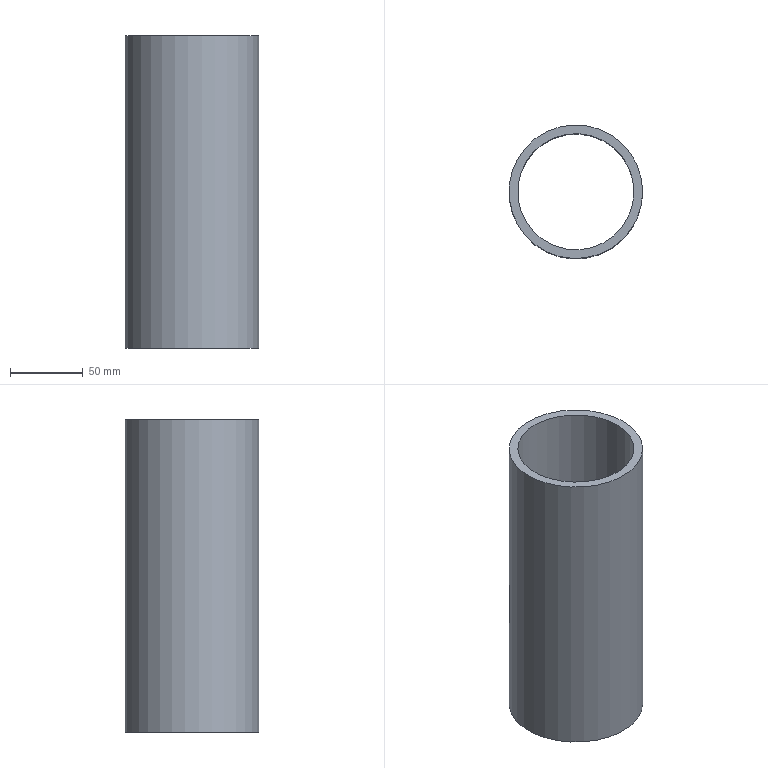Part | STEP file | lll_id2866_x_t | 1 solid | 4 faces | box 92 x 92 x 215 mm | volume 348528 mm3 | cylinder 2 | plane 2 | commonest cylinder face diameters 80 x1 92 x1
STEP:
#1=CARTESIAN_POINT('',(498.435,500.,-329.5));
#2=VERTEX_POINT('',#1);
#3=CARTESIAN_POINT('',(452.435,500.,-329.5));
#4=DIRECTION('',(0.,0.,-1.));
#5=DIRECTION('',(1.,0.,0.));
#6=AXIS2_PLACEMENT_3D('',#3,#4,#5);
#7=CIRCLE('',#6,46.);
#8=EDGE_CURVE('',#2,#2,#7,.T.);
#9=ORIENTED_EDGE('',*,*,#8,.F.);
#10=EDGE_LOOP('',(#9));
#11=FACE_BOUND('',#10,.T.);
#12=CARTESIAN_POINT('',(498.435,500.,-114.5));
#13=VERTEX_POINT('',#12);
#14=CARTESIAN_POINT('',(452.435,500.,-114.5));
#15=DIRECTION('',(0.,0.,-1.));
#16=DIRECTION('',(1.,0.,0.));
#17=AXIS2_PLACEMENT_3D('',#14,#15,#16);
#18=CIRCLE('',#17,46.);
#19=EDGE_CURVE('',#13,#13,#18,.T.);
#20=ORIENTED_EDGE('',*,*,#19,.T.);
#21=EDGE_LOOP('',(#20));
#22=FACE_BOUND('',#21,.T.);
#23=CARTESIAN_POINT('',(452.435,500.,-329.5));
#24=DIRECTION('',(0.,0.,1.));
#25=DIRECTION('',(1.,0.,0.));
#26=AXIS2_PLACEMENT_3D('',#23,#24,#25);
#27=CYLINDRICAL_SURFACE('',#26,46.);
#28=ADVANCED_FACE('',(#11,#22),#27,.T.);
#29=CARTESIAN_POINT('',(492.435,500.,-329.5));
#30=VERTEX_POINT('',#29);
#31=CARTESIAN_POINT('',(452.435,500.,-329.5));
#32=DIRECTION('',(0.,0.,-1.));
#33=DIRECTION('',(1.,0.,0.));
#34=AXIS2_PLACEMENT_3D('',#31,#32,#33);
#35=CIRCLE('',#34,40.);
#36=EDGE_CURVE('',#30,#30,#35,.T.);
#37=ORIENTED_EDGE('',*,*,#36,.T.);
#38=EDGE_LOOP('',(#37));
#39=FACE_BOUND('',#38,.T.);
#40=CARTESIAN_POINT('',(492.435,500.,-114.5));
#41=VERTEX_POINT('',#40);
#42=CARTESIAN_POINT('',(452.435,500.,-114.5));
#43=DIRECTION('',(0.,0.,-1.));
#44=DIRECTION('',(1.,0.,0.));
#45=AXIS2_PLACEMENT_3D('',#42,#43,#44);
#46=CIRCLE('',#45,40.);
#47=EDGE_CURVE('',#41,#41,#46,.T.);
#48=ORIENTED_EDGE('',*,*,#47,.F.);
#49=EDGE_LOOP('',(#48));
#50=FACE_BOUND('',#49,.T.);
#51=CARTESIAN_POINT('',(452.435,500.,-329.5));
#52=DIRECTION('',(0.,0.,1.));
#53=DIRECTION('',(1.,0.,0.));
#54=AXIS2_PLACEMENT_3D('',#51,#52,#53);
#55=CYLINDRICAL_SURFACE('',#54,40.);
#56=ADVANCED_FACE('',(#39,#50),#55,.F.);
#57=ORIENTED_EDGE('',*,*,#8,.T.);
#58=EDGE_LOOP('',(#57));
#59=FACE_BOUND('',#58,.T.);
#60=ORIENTED_EDGE('',*,*,#36,.F.);
#61=EDGE_LOOP('',(#60));
#62=FACE_BOUND('',#61,.T.);
#63=CARTESIAN_POINT('',(452.435,500.,-329.5));
#64=DIRECTION('',(0.,0.,1.));
#65=DIRECTION('',(1.,0.,0.));
#66=AXIS2_PLACEMENT_3D('',#63,#64,#65);
#67=PLANE('',#66);
#68=ADVANCED_FACE('',(#59,#62),#67,.F.);
#69=ORIENTED_EDGE('',*,*,#19,.F.);
#70=EDGE_LOOP('',(#69));
#71=FACE_BOUND('',#70,.T.);
#72=ORIENTED_EDGE('',*,*,#47,.T.);
#73=EDGE_LOOP('',(#72));
#74=FACE_BOUND('',#73,.T.);
#75=CARTESIAN_POINT('',(452.435,500.,-114.5));
#76=DIRECTION('',(0.,0.,1.));
#77=DIRECTION('',(1.,0.,0.));
#78=AXIS2_PLACEMENT_3D('',#75,#76,#77);
#79=PLANE('',#78);
#80=ADVANCED_FACE('',(#71,#74),#79,.T.);
#81=CLOSED_SHELL('',(#28,#56,#68,#80));
#82=MANIFOLD_SOLID_BREP('',#81);
#83=(LENGTH_UNIT()NAMED_UNIT(*)SI_UNIT(.MILLI.,.METRE.));
#84=UNCERTAINTY_MEASURE_WITH_UNIT(LENGTH_MEASURE(0.00002),#83,'','');
#85=(NAMED_UNIT(*)PLANE_ANGLE_UNIT()SI_UNIT($,.RADIAN.));
#86=PLANE_ANGLE_MEASURE_WITH_UNIT(PLANE_ANGLE_MEASURE(0.01745),#85);
#87=DIMENSIONAL_EXPONENTS(0.,0.,0.,0.,0.,0.,0.);
#88=(CONVERSION_BASED_UNIT('DEGREE',#86)NAMED_UNIT(#87)PLANE_ANGLE_UNIT());
#89=(NAMED_UNIT(*)SI_UNIT($,.STERADIAN.)SOLID_ANGLE_UNIT());
#90=(GEOMETRIC_REPRESENTATION_CONTEXT(3)GLOBAL_UNCERTAINTY_ASSIGNED_CONTEXT((#84))GLOBAL_UNIT_ASSIGNED_CONTEXT((#83,#88,#89))REPRESENTATION_CONTEXT('',''));
#91=ADVANCED_BREP_SHAPE_REPRESENTATION('',(#82),#90);